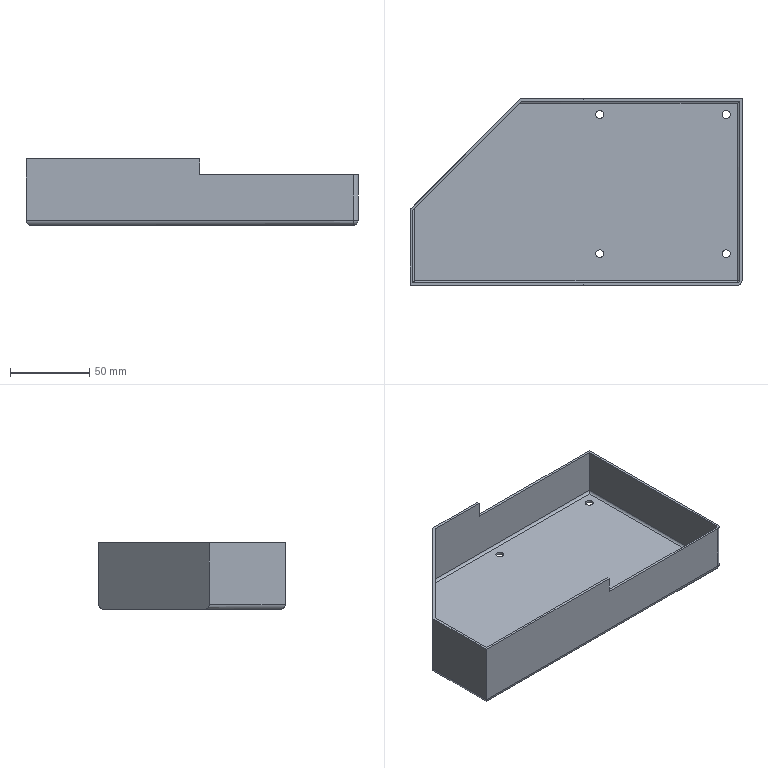Part | STEP file | PN_0009_default[machined] | 1 solid | 36 faces | box 210 x 118 x 42 mm | volume 64871 mm3 | cylinder 18 | plane 16 | sphere 2 | commonest cylinder face diameters 5 x8 3 x5 6 x5